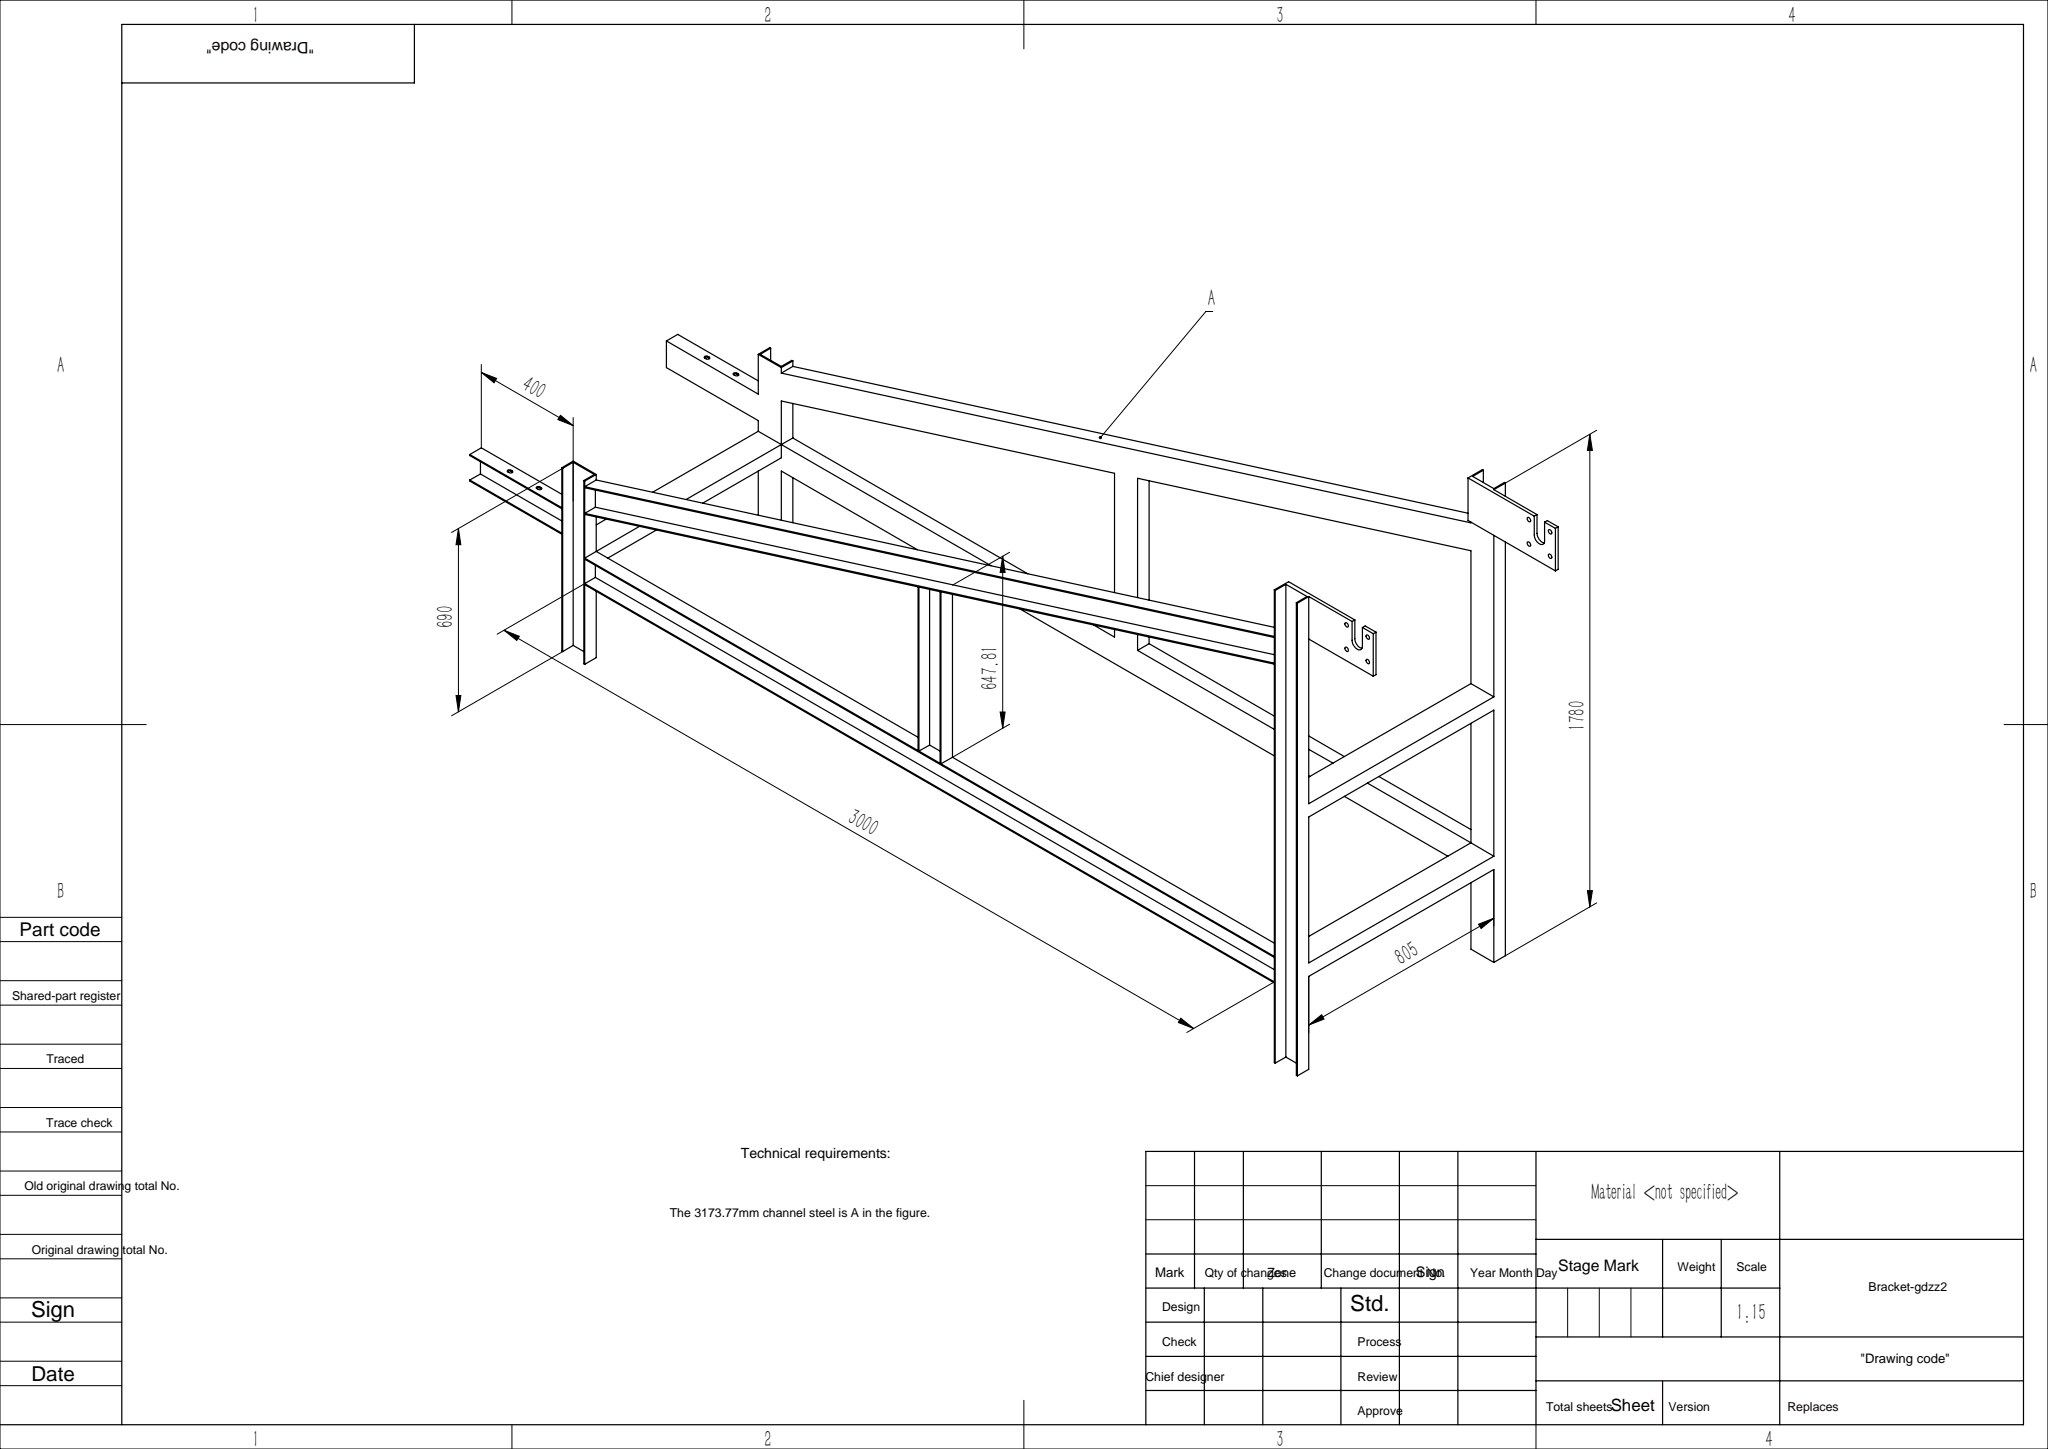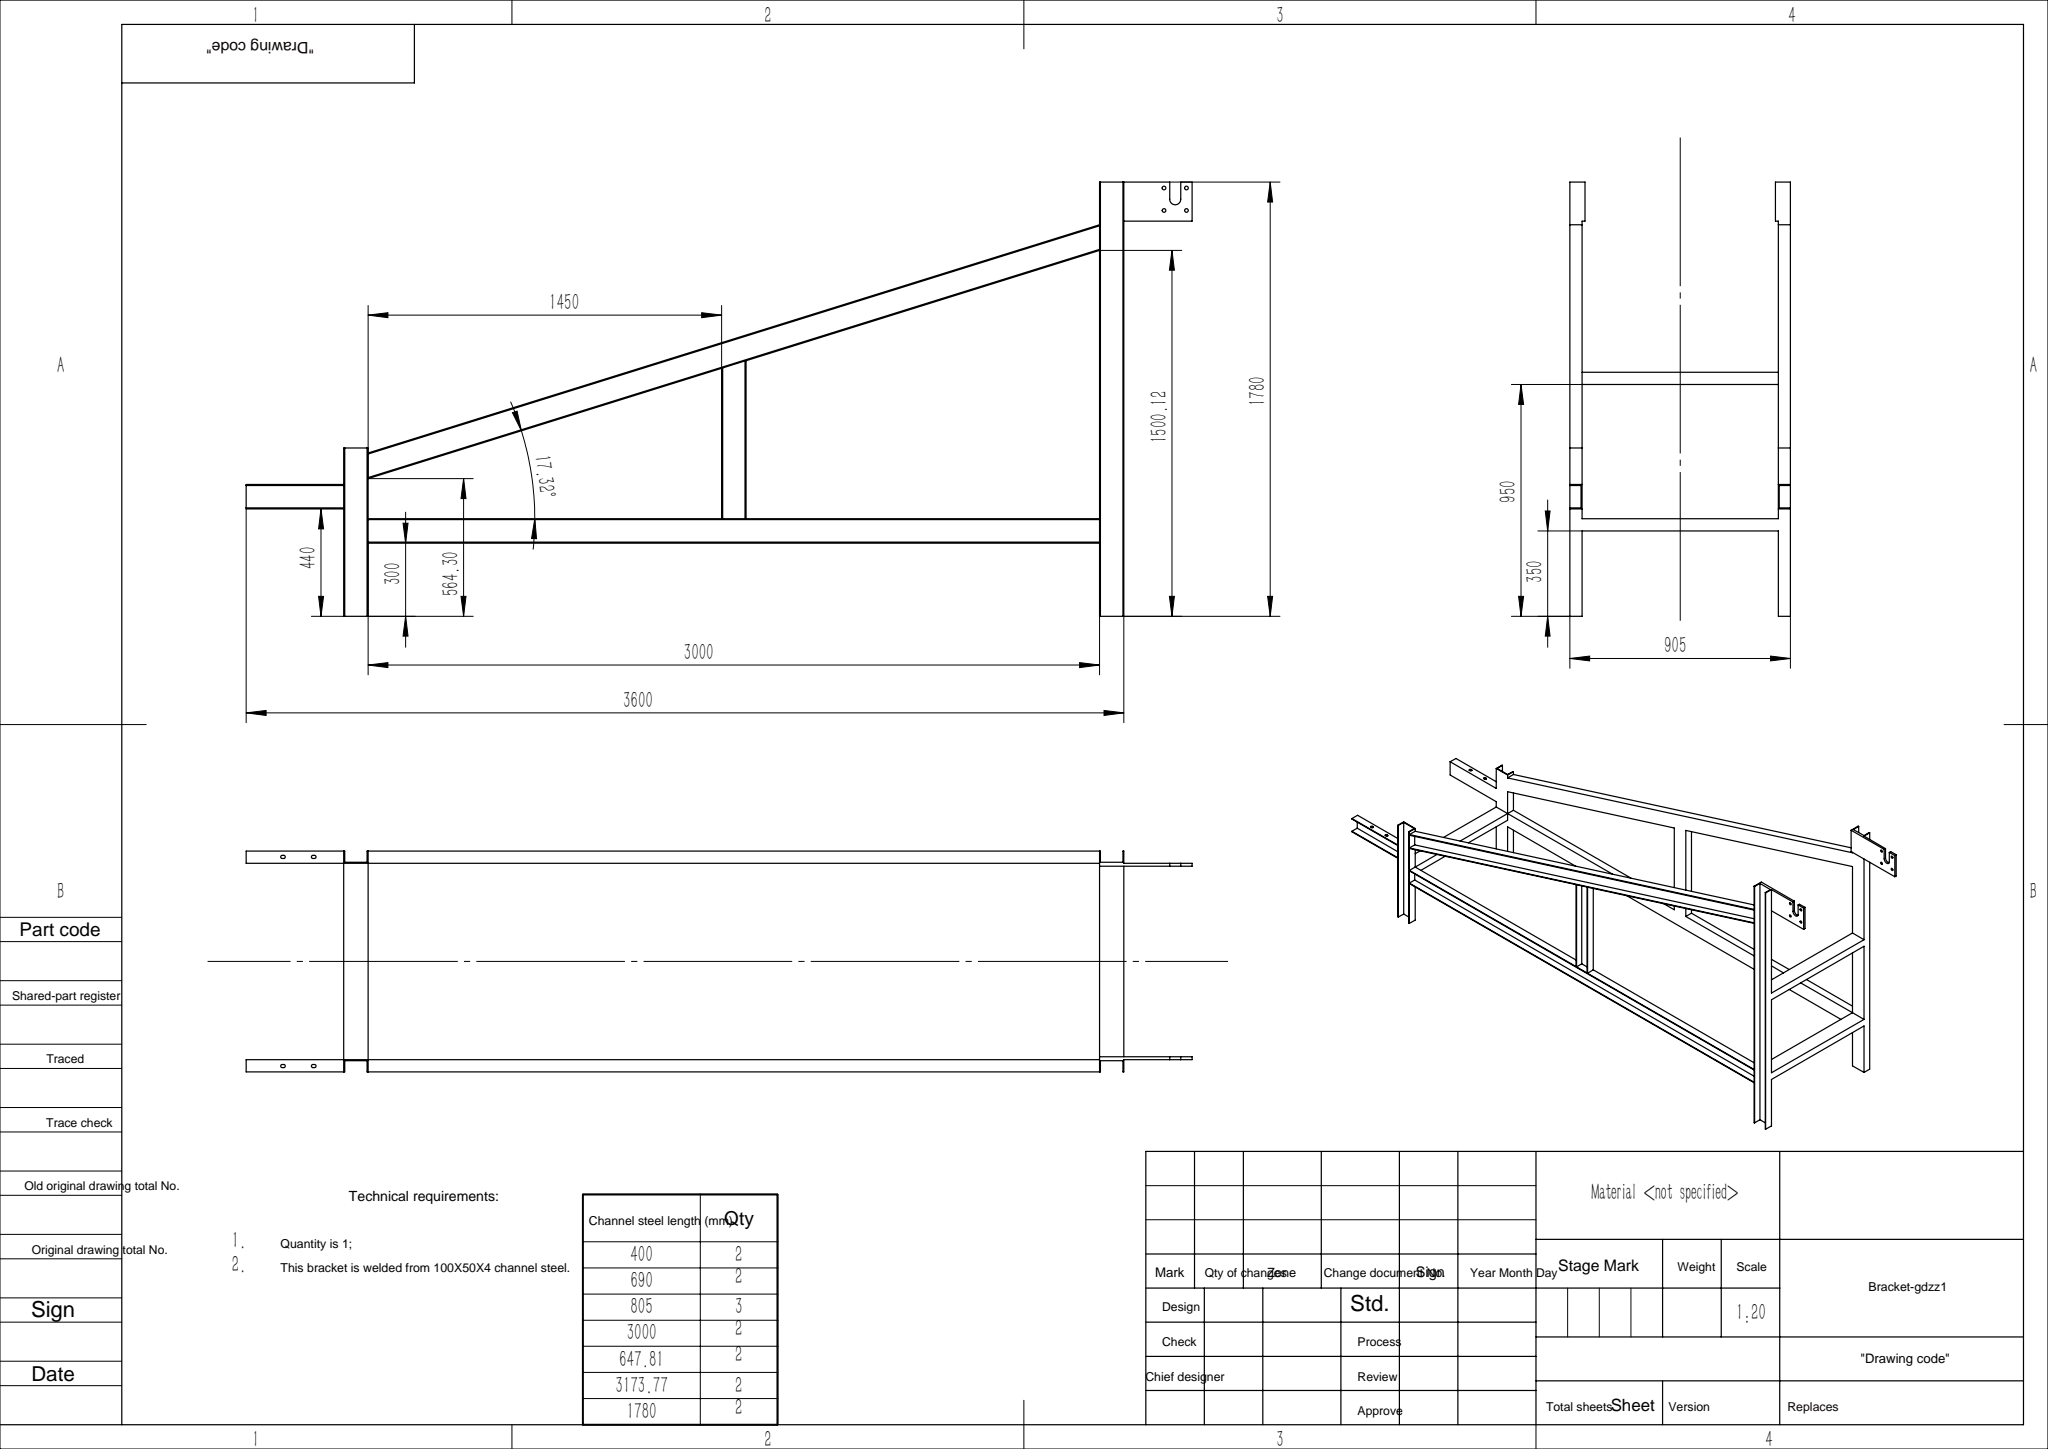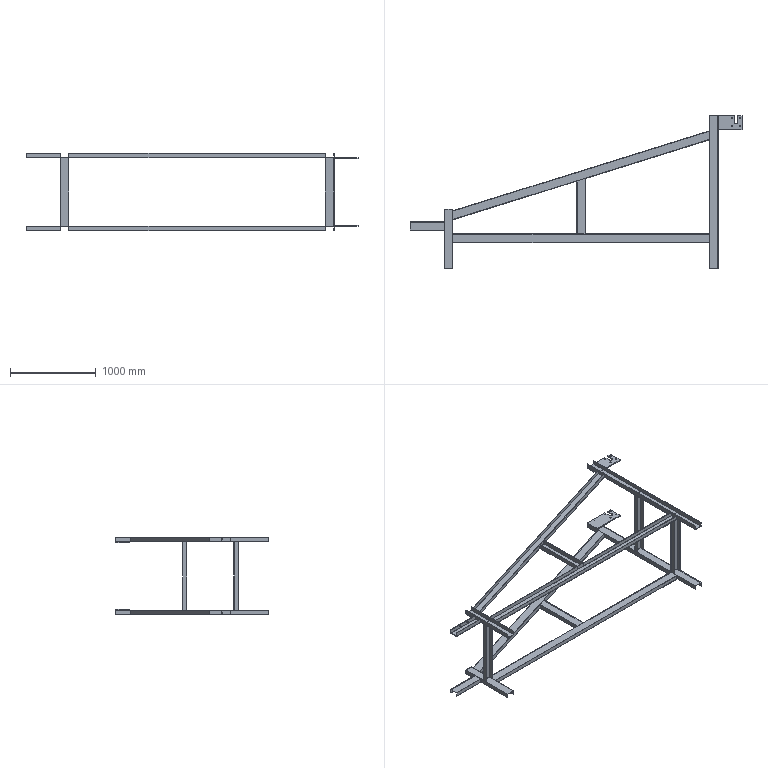Part | SolidWorks | features ICE 8, Cut 3, MirrorPattern 3, Extrusion 1, LPattern 1 | 1 solid | 173 faces | box 3880 x 1780 x 905 mm | volume 18012747 mm3 | plane 147 | cylinder 26 | commonest cylinder face diameters 15 x16 13 x8 45 x2